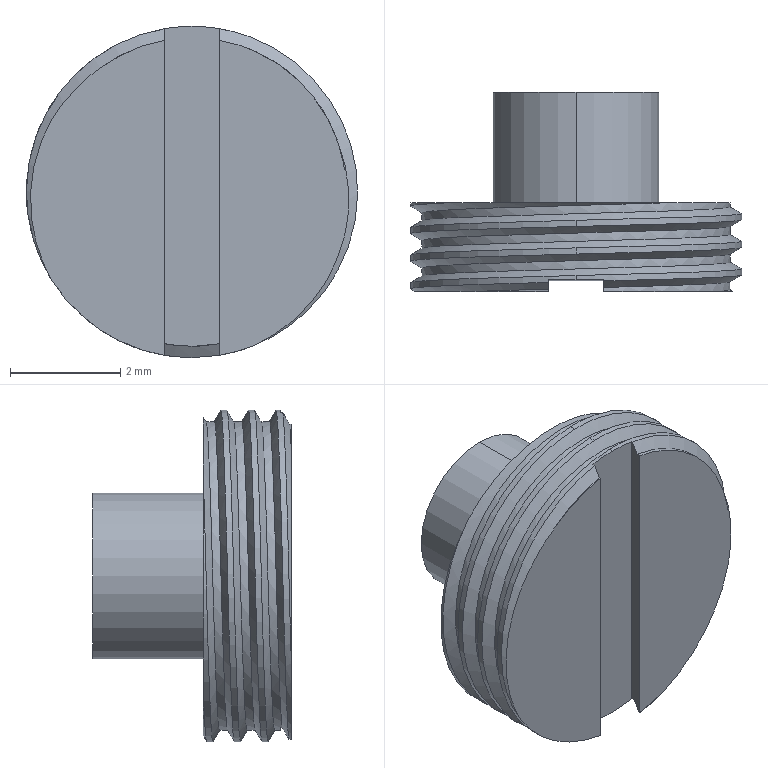Part | SolidWorks | features ICE 2, Extrusion 1, Helix 1, SweepCut 1 | 1 solid | 23 faces | box 6 x 3.6 x 6 mm | volume 54.971 mm3 | cylinder 10 | plane 7 | spline 6 | commonest cylinder face diameters 6 x8 3 x2